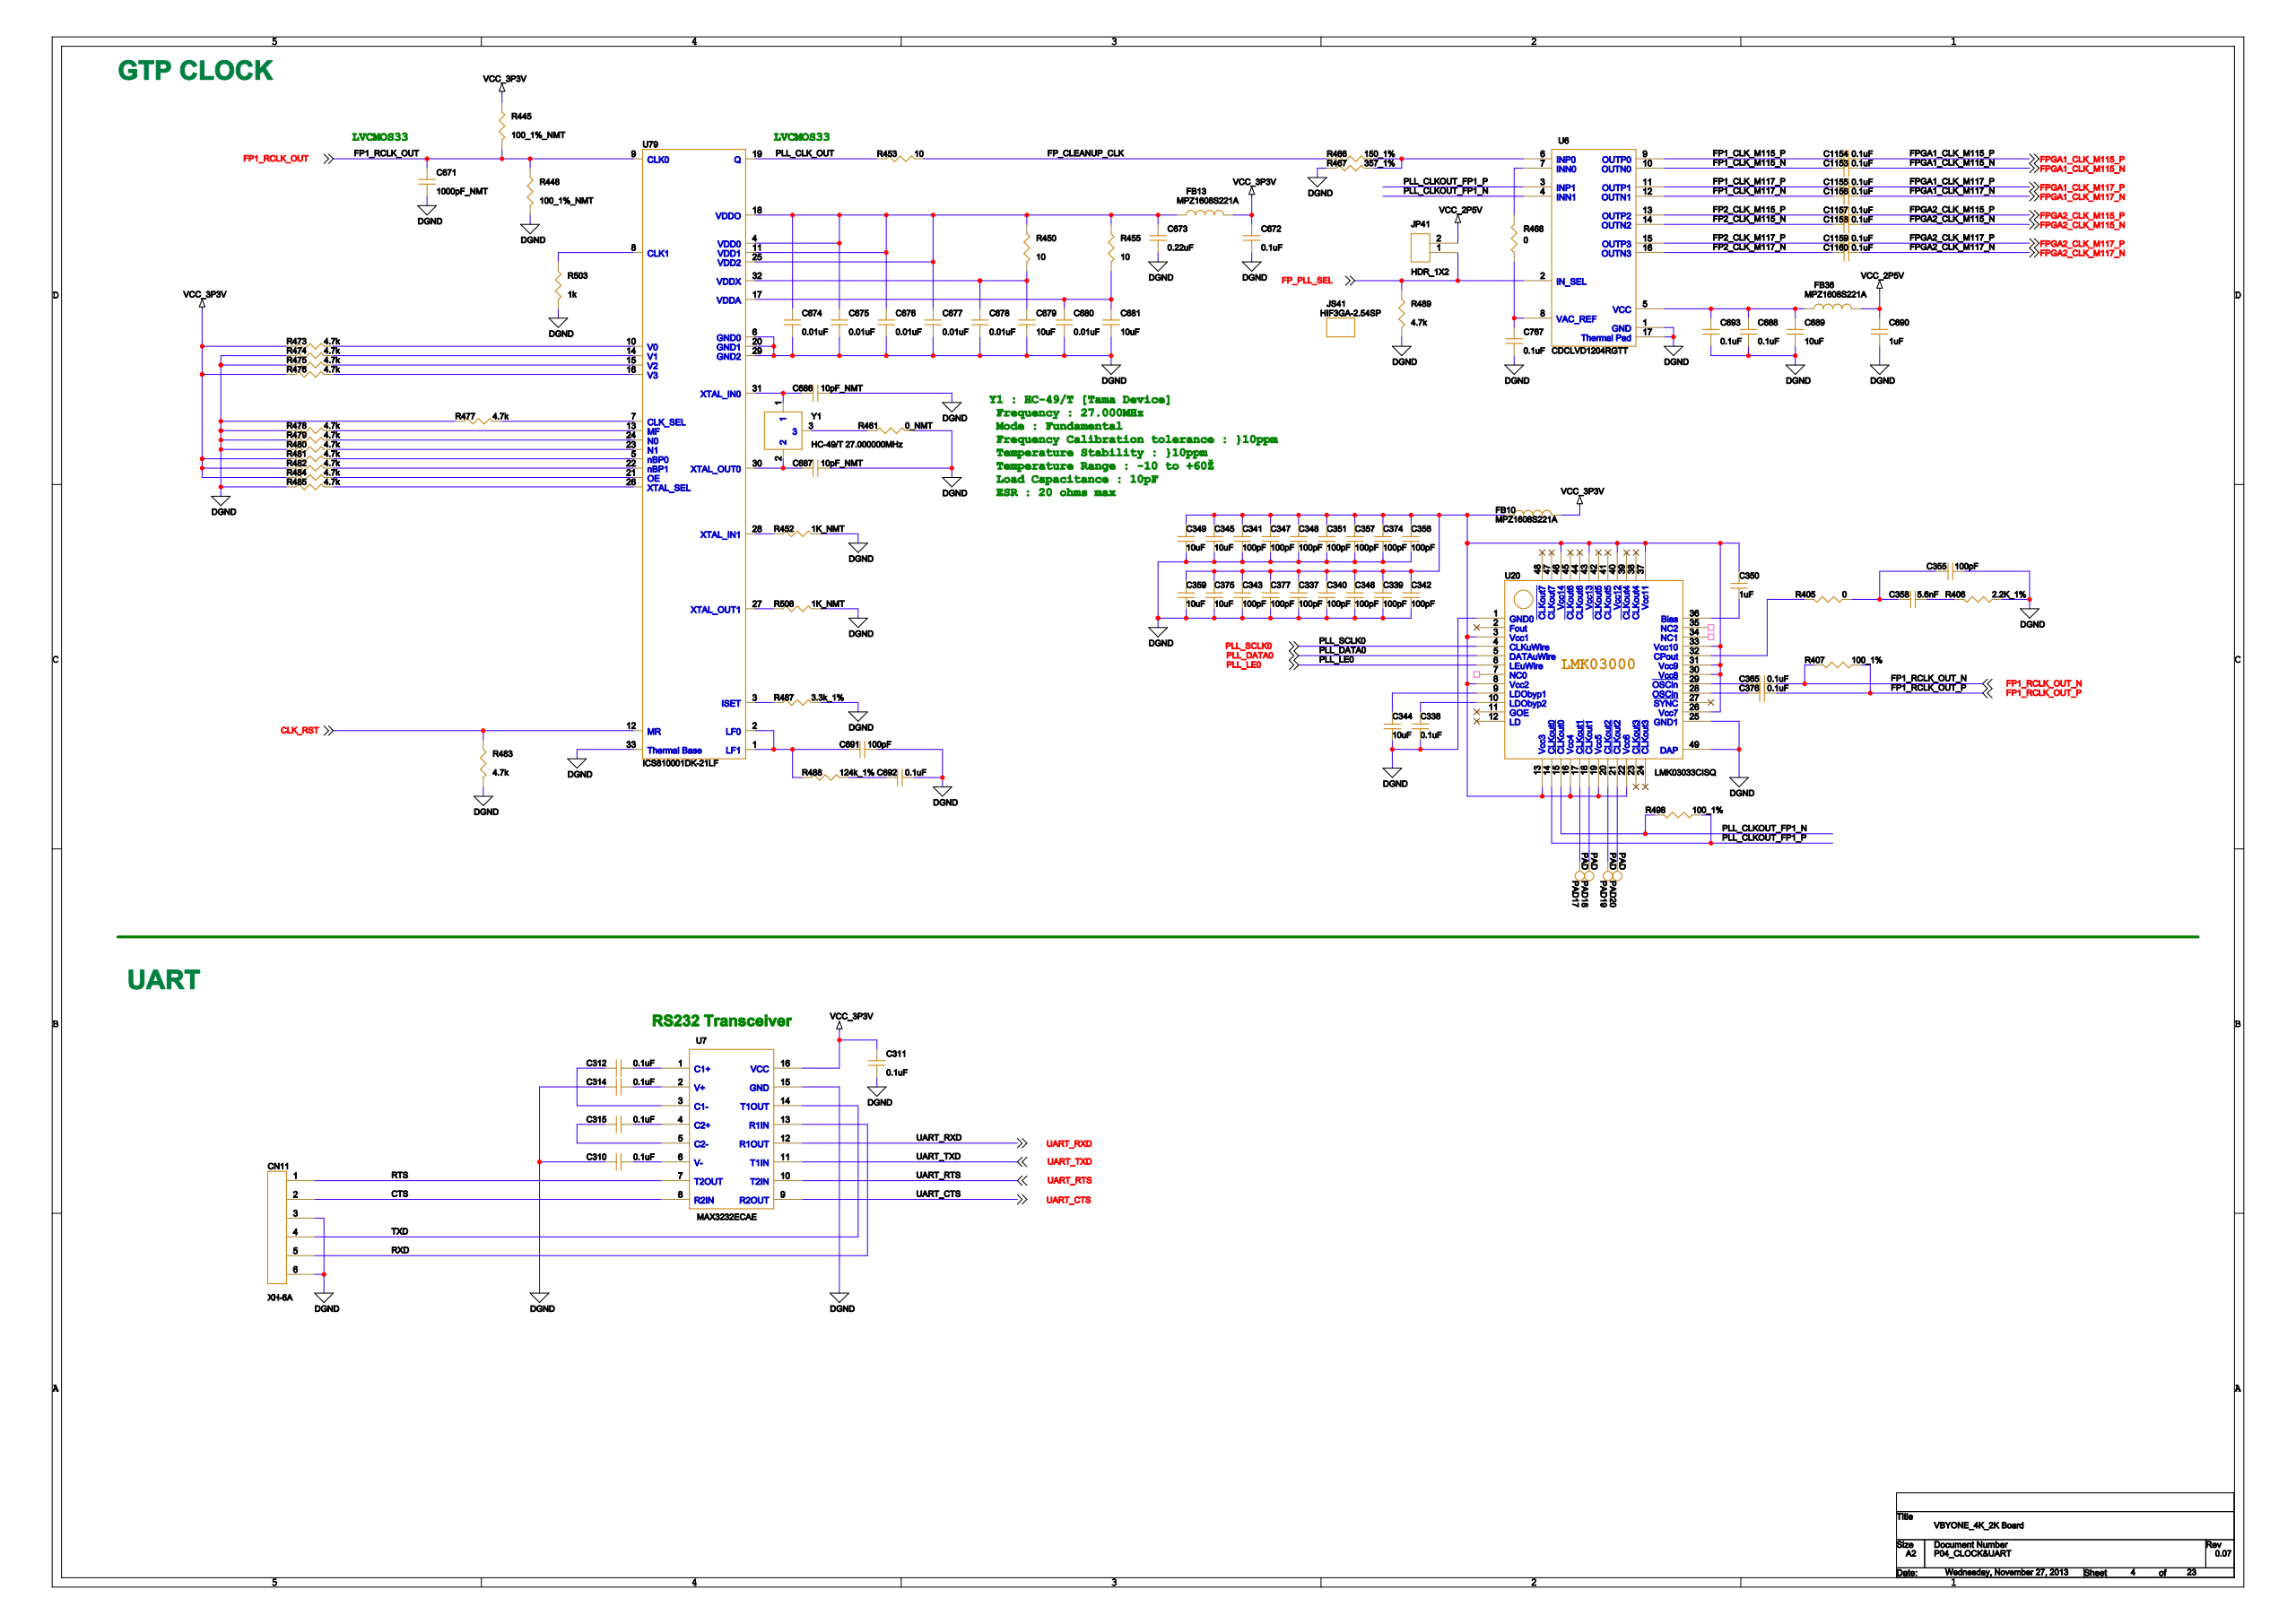Circuit board | Cadence Allegro | 1712 parts | 1495 nets | one sheet of the schematic
Parts on this sheet (reference | value | footprint):
C310 | 0.1uF | CRC1005RZAS
C311 | 0.1uF | CRC1005RZAS
C312 | 0.1uF | CRC1005RZAS
C314 | 0.1uF | CRC1005RZAS
C315 | 0.1uF | CRC1005RZAS
C337 | 100pF | CRC1608RZAS
C338 | 0.1uF | CRC1005RZAS
C339 | 100pF | CRC1608RZAS
C340 | 100pF | CRC1608RZAS
C341 | 100pF | CRC1608RZAS
C342 | 100pF | CRC1608RZAS
C343 | 100pF | CRC1608RZAS
C344 | 10uF | CRC2012RZAS
C345 | 10uF | CRC2012RZAS
C346 | 100pF | CRC1608RZAS
C347 | 100pF | CRC1608RZAS
C348 | 100pF | CRC1608RZAS
C349 | 10uF | CRC2012RZAS
C350 | 1uF | CRC1608RZAS
C351 | 100pF | CRC1608RZAS
C355 | 100pF | CRC1608RZAS
C356 | 100pF | CRC1608RZAS
C357 | 100pF | CRC1608RZAS
C358 | 5.6nF | CRC1608RZAS
C359 | 10uF | CRC2012RZAS
C365 | 0.1uF | CRC1005RZAS
C374 | 100pF | CRC1608RZAS
C375 | 10uF | CRC2012RZAS
C376 | 0.1uF | CRC1005RZAS
C377 | 100pF | CRC1608RZAS
C671 | 1000pF_NMT | CRC1608RZAS
C672 | 0.1uF | CRC1005RZAS
C673 | 0.22uF | CRC1608RZAS
C674 | 0.01uF | CRC1005RZAS
C675 | 0.01uF | CRC1005RZAS
C676 | 0.01uF | CRC1005RZAS
C677 | 0.01uF | CRC1005RZAS
C678 | 0.01uF | CRC1005RZAS
C679 | 10uF | CRC2012RZAS
C680 | 0.01uF | CRC1005RZAS
C681 | 10uF | CRC2012RZAS
C686 | 10pF_NMT | CRC1608RZAS
C687 | 10pF_NMT | CRC1608RZAS
C688 | 0.1uF | CRC1005RZAS
C689 | 10uF | CRC2012RZAS
C690 | 1uF | CRC1608RZAS
C691 | 100pF | CRC1608RZAS
C692 | 0.1uF | CRC1005RZAS
C693 | 0.1uF | CRC1005RZAS
C767 | 0.1uF | CRC1005RZAS
C1153 | 0.1uF | CRC1005RZAS
C1154 | 0.1uF | CRC1005RZAS
C1155 | 0.1uF | CRC1005RZAS
C1156 | 0.1uF | CRC1005RZAS
C1157 | 0.1uF | CRC1005RZAS
C1158 | 0.1uF | CRC1005RZAS
C1159 | 0.1uF | CRC1005RZAS
C1160 | 0.1uF | CRC1005RZAS
CN11 | XH-6A | CND006LKAS
FB10 | MPZ1608S221A | LSC1608RZAS
FB13 | MPZ1608S221A | LSC1608RZAS
FB36 | MPZ1608S221A | LSC1608RZAS
JP41 | HDR_1X2 | CND002LLBS
PAD17 | PAD | TPC050
PAD18 | PAD | TPC050
PAD19 | PAD | TPC050
PAD20 | PAD | TPC050
R405 | 0 | CRC1608RZAS
R406 | 2.2K_1% | CRC1005RZAS
R407 | 100_1% | CRC1005RZAS
R445 | 100_1%_NMT | CRC1608RZAS
R448 | 100_1%_NMT | CRC1608RZAS
R450 | 10 | CRC1005RZAS
R452 | 1K_NMT | CRC1608RZAS
R453 | 10 | CRC1005RZAS
R455 | 10 | CRC1005RZAS
R461 | 0_NMT | CRC1608RZAS
R466 | 150_1% | CRC1608RZAS
R467 | 357_1% | CRC1608RZAS
R468 | 0 | CRC1608RZAS
R473 | 4.7K | CRC1005RZAS
R474 | 4.7K | CRC1005RZAS
R475 | 4.7K | CRC1005RZAS
R476 | 4.7K | CRC1005RZAS
R477 | 4.7K | CRC1005RZAS
R478 | 4.7K | CRC1005RZAS
R479 | 4.7K | CRC1005RZAS
R480 | 4.7K | CRC1005RZAS
R481 | 4.7K | CRC1005RZAS
R482 | 4.7K | CRC1005RZAS
R483 | 4.7K | CRC1005RZAS
R484 | 4.7K | CRC1005RZAS
R485 | 4.7K | CRC1005RZAS
R487 | 3.3k_1% | CRC1608RZAS
R488 | 124k_1% | CRC1608RZAS
R489 | 4.7K | CRC1005RZAS
R498 | 100_1% | CRC1005RZAS
R503 | 1k | CRC1608RZAS
R508 | 1K_NMT | CRC1608RZAS
U6 | CDCLVD1204RGTT | QFN016RCAS
U7 | MAX3232ECAE | SOC016REDS
U20 | LMK03033CISQ | QFN048RCBS
U79 | ICS810001DK-21LF | QFN032RCBS
Nets of these parts (net: part-pin ...):
VCC_3P3V: C311-1 C672-1 FB10-2 FB13-2 R445-1 R473-1 R476-1 R481-1 R482-1 R484-1 U7-16
DGND: C310-1 C311-2 C314-1 C337-1 C338-1 C339-1 C340-1 C341-1 C342-1 C343-1 C344-1 C345-1 C346-1 C347-1 C348-1 C349-1 C351-1 C355-1 C356-1 C357-1 C359-1 C374-1 C375-1 C377-1 C671-2 C672-2 C673-2 C674-2 C675-2 C676-2 C677-2 C678-2 C679-2 C680-2 C681-2 C686-2 C687-2 C688-2 C689-2 C690-2 C691-2 C692-2 C693-2 C767-2 CN11-3 CN11-6 R406-1 R448-2 R452-2 R461-2 R467-1 R474-1 R475-1 R477-1 R478-1 R479-1 R480-1 R483-2 R485-1 R487-2 R489-2 R503-2 R508-2 U6-1 U6-17 U7-15 U20-1 U20-25 U20-49 U79-6 U79-20 U79-29 U79-33
VCC_2P5V: C690-1 FB36-2 JP41-2
FP1_CLK_M115_N: C1153-1 U6-10
FPGA1_CLK_M115_N: C1153-2
FP1_CLK_M115_P: C1154-1 U6-9
FPGA1_CLK_M115_P: C1154-2
FP1_CLK_M117_P: C1155-1 U6-11
FPGA1_CLK_M117_P: C1155-2
FP1_CLK_M117_N: C1156-1 U6-12
FPGA1_CLK_M117_N: C1156-2
FP2_CLK_M115_P: C1157-1 U6-13
FPGA2_CLK_M115_P: C1157-2
FP2_CLK_M115_N: C1158-1 U6-14
FPGA2_CLK_M115_N: C1158-2
FP2_CLK_M117_P: C1159-1 U6-15
FPGA2_CLK_M117_P: C1159-2
FP2_CLK_M117_N: C1160-1 U6-16
FPGA2_CLK_M117_N: C1160-2
N18371035: C688-1 C689-1 C693-1 FB36-1 U6-5
N17909593: C692-1 R488-2
N18370724: C767-1 R468-1 U6-8
N17910053: C678-1 C679-1 R450-2 U79-32
N17910049: C680-1 C681-1 R455-2 U79-17
N19016279: C344-2 U20-9
N19016231: C337-2 C339-2 C340-2 C341-2 C342-2 C343-2 C345-2 C346-2 C347-2 C348-2 C349-2 C350-2 C351-2 C356-2 C357-2 C359-2 C374-2 C375-2 C377-2 FB10-1 U20-3 U20-8 U20-13 U20-16 U20-19 U20-22 U20-26 U20-30 U20-31 U20-33 U20-37 U20-40 U20-43 U20-46
N17910041: C673-1 C674-1 C675-1 C676-1 C677-1 FB13-1 R450-1 R455-1 U79-4 U79-11 U79-18 U79-25
N19221929: C310-2 U7-6
N19221949: C312-1 U7-3
N19221955: C312-2 U7-1
N19221931: C314-2 U7-2
N19221941: C315-1 U7-5
N19221947: C315-2 U7-4
N19016269: C338-2 U20-10
N19016656: C365-1 U20-29
FP1_RCLK_OUT_N: C365-2 R407-2
N19016658: C376-1 U20-28
FP1_RCLK_OUT_P: C376-2 R407-1
N19016493: C355-2 C358-2 R405-1
N19016353: C350-1 U20-36
N19016582: C358-1 R406-2
FP1_RCLK_OUT: C671-1 R445-2 R448-1 U79-9
N17910001: C686-1 U79-31
N17909989: C687-1 U79-30
N17909569: C691-1 R488-1 U79-1 U79-2
RTS: CN11-1 U7-7
CTS: CN11-2 U7-8
TXD: CN11-4 U7-14
RXD: CN11-5 U7-13
FP_PLL_SEL: JP41-1 R489-1 U6-2
N19385728: PAD17-1 U20-17
N19385772: PAD18-1 U20-18
N19385776: PAD19-1 U20-20
N19385787: PAD20-1 U20-21
N19016578: R405-2 U20-32
N18370679: R468-2 U6-7
PLL_CLKOUT_FP1_P: R498-1 U6-3 U20-14
PLL_CLKOUT_FP1_N: R498-2 U6-4 U20-15
N17909971: R473-2 U79-10
N17909969: R474-2 U79-14
N17909973: R475-2 U79-15
N17909967: R476-2 U79-16
N17909914: R477-2 U79-7
N17909955: R478-2 U79-13
N17909953: R479-2 U79-24
N17909951: R480-2 U79-23
N17909947: R481-2 U79-5
N17909943: R482-2 U79-22
CLK_RST: R483-1 U79-12
N17909931: R484-2 U79-21
N17909900: R485-2 U79-26
N20610566: R461-1
N17909621: R452-1 U79-28
N17909646: R508-1 U79-27
PLL_CLK_OUT: R453-1 U79-19
FP_CLEANUP_CLK: R453-2 R466-1
N18371118: R466-2 R467-2 U6-6
N17909602: R487-1 U79-3
N18373017: R503-1 U79-8
UART_RXD: U7-12
PLL_SCLK0: U20-4
UART_TXD: U7-11
PLL_LE0: U20-6
PLL_DATA0: U20-5
UART_CTS: U7-9
UART_RTS: U7-10